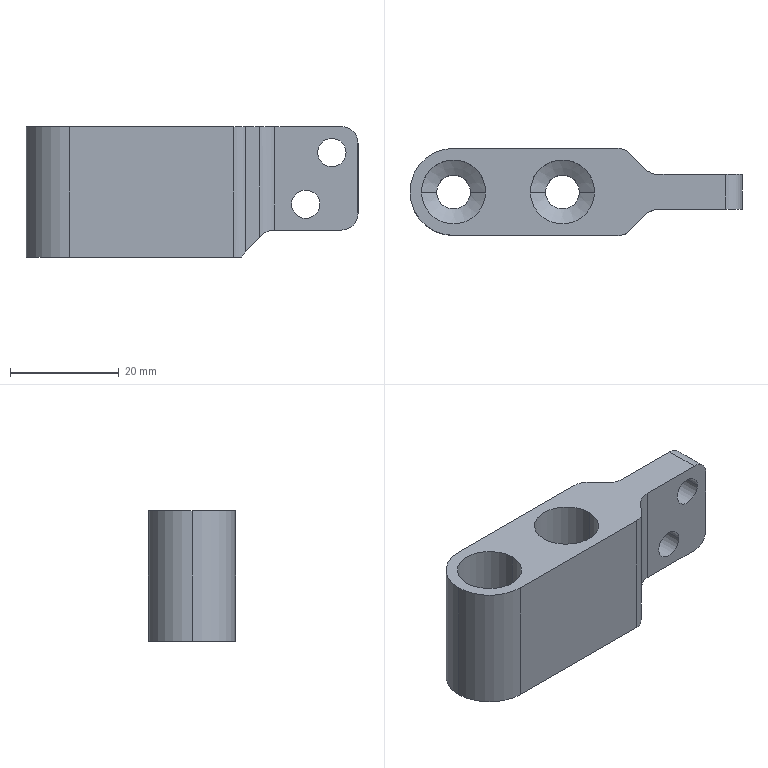Part | NX | 1 solid | 36 faces | box 60.988 x 16 x 24 mm | volume 13127 mm3 | cylinder 21 | plane 11 | cone 4 | commonest cylinder face diameters 5.2 x4 6 x4 6.2 x4 11.8 x4 8 x3 16 x2
STEP:
#1=CARTESIAN_POINT('',(-16.594,0.,-17.));
#2=VERTEX_POINT('',#1);
#3=CARTESIAN_POINT('',(-28.394,0.,-17.));
#4=VERTEX_POINT('',#3);
#5=CARTESIAN_POINT('',(-22.494,0.,-17.));
#6=DIRECTION('',(0.,0.,1.));
#7=DIRECTION('',(-1.,0.,0.));
#8=AXIS2_PLACEMENT_3D('',#5,#6,#7);
#9=CIRCLE('',#8,5.9);
#10=EDGE_CURVE('',#2,#4,#9,.T.);
#11=ORIENTED_EDGE('',*,*,#10,.F.);
#12=CARTESIAN_POINT('',(-16.594,0.,0.));
#13=VERTEX_POINT('',#12);
#14=CARTESIAN_POINT('',(-16.594,0.,0.));
#15=DIRECTION('',(0.,0.,1.));
#16=VECTOR('',#15,1000.);
#17=LINE('',#14,#16);
#18=EDGE_CURVE('',#13,#2,#17,.F.);
#19=ORIENTED_EDGE('',*,*,#18,.F.);
#20=CARTESIAN_POINT('',(-28.394,0.,0.));
#21=VERTEX_POINT('',#20);
#22=CARTESIAN_POINT('',(-22.494,0.,0.));
#23=DIRECTION('',(0.,0.,1.));
#24=DIRECTION('',(-1.,0.,0.));
#25=AXIS2_PLACEMENT_3D('',#22,#23,#24);
#26=CIRCLE('',#25,5.9);
#27=EDGE_CURVE('',#13,#21,#26,.T.);
#28=ORIENTED_EDGE('',*,*,#27,.T.);
#29=CARTESIAN_POINT('',(-28.394,0.,0.));
#30=DIRECTION('',(0.,0.,1.));
#31=VECTOR('',#30,1000.);
#32=LINE('',#29,#31);
#33=EDGE_CURVE('',#21,#4,#32,.F.);
#34=ORIENTED_EDGE('',*,*,#33,.T.);
#35=EDGE_LOOP('',(#11,#19,#28,#34));
#36=FACE_BOUND('',#35,.T.);
#37=CARTESIAN_POINT('',(-22.494,0.,0.));
#38=DIRECTION('',(0.,0.,1.));
#39=DIRECTION('',(1.,0.,0.));
#40=AXIS2_PLACEMENT_3D('',#37,#38,#39);
#41=CYLINDRICAL_SURFACE('',#40,5.9);
#42=ADVANCED_FACE('',(#36),#41,.F.);
#43=CARTESIAN_POINT('',(-19.394,0.,-18.682));
#44=VERTEX_POINT('',#43);
#45=CARTESIAN_POINT('',(-25.594,0.,-18.682));
#46=VERTEX_POINT('',#45);
#47=CARTESIAN_POINT('',(-22.494,0.,-18.682));
#48=DIRECTION('',(0.,0.,1.));
#49=DIRECTION('',(-1.,0.,0.));
#50=AXIS2_PLACEMENT_3D('',#47,#48,#49);
#51=CIRCLE('',#50,3.1);
#52=EDGE_CURVE('',#44,#46,#51,.T.);
#53=ORIENTED_EDGE('',*,*,#52,.F.);
#54=CARTESIAN_POINT('',(-16.594,0.,-17.));
#55=DIRECTION('',(0.8572,0.,0.515));
#56=VECTOR('',#55,1000.);
#57=LINE('',#54,#56);
#58=EDGE_CURVE('',#2,#44,#57,.F.);
#59=ORIENTED_EDGE('',*,*,#58,.F.);
#60=ORIENTED_EDGE('',*,*,#10,.T.);
#61=CARTESIAN_POINT('',(-28.394,0.,-17.));
#62=DIRECTION('',(-0.8572,0.,0.515));
#63=VECTOR('',#62,1000.);
#64=LINE('',#61,#63);
#65=EDGE_CURVE('',#4,#46,#64,.F.);
#66=ORIENTED_EDGE('',*,*,#65,.T.);
#67=EDGE_LOOP('',(#53,#59,#60,#66));
#68=FACE_BOUND('',#67,.T.);
#69=CARTESIAN_POINT('',(-22.494,0.,-17.));
#70=DIRECTION('',(0.,0.,1.));
#71=DIRECTION('',(1.,0.,0.));
#72=AXIS2_PLACEMENT_3D('',#69,#70,#71);
#73=CONICAL_SURFACE('',#72,5.9,1.03);
#74=ADVANCED_FACE('',(#68),#73,.F.);
#75=CARTESIAN_POINT('',(3.406,0.,-17.));
#76=VERTEX_POINT('',#75);
#77=CARTESIAN_POINT('',(-8.394,0.,-17.));
#78=VERTEX_POINT('',#77);
#79=CARTESIAN_POINT('',(-2.494,0.,-17.));
#80=DIRECTION('',(0.,0.,1.));
#81=DIRECTION('',(-1.,0.,0.));
#82=AXIS2_PLACEMENT_3D('',#79,#80,#81);
#83=CIRCLE('',#82,5.9);
#84=EDGE_CURVE('',#76,#78,#83,.T.);
#85=ORIENTED_EDGE('',*,*,#84,.F.);
#86=CARTESIAN_POINT('',(3.406,0.,0.));
#87=VERTEX_POINT('',#86);
#88=CARTESIAN_POINT('',(3.406,0.,0.));
#89=DIRECTION('',(0.,0.,1.));
#90=VECTOR('',#89,1000.);
#91=LINE('',#88,#90);
#92=EDGE_CURVE('',#87,#76,#91,.F.);
#93=ORIENTED_EDGE('',*,*,#92,.F.);
#94=CARTESIAN_POINT('',(-8.394,0.,0.));
#95=VERTEX_POINT('',#94);
#96=CARTESIAN_POINT('',(-2.494,0.,0.));
#97=DIRECTION('',(0.,0.,1.));
#98=DIRECTION('',(-1.,0.,0.));
#99=AXIS2_PLACEMENT_3D('',#96,#97,#98);
#100=CIRCLE('',#99,5.9);
#101=EDGE_CURVE('',#87,#95,#100,.T.);
#102=ORIENTED_EDGE('',*,*,#101,.T.);
#103=CARTESIAN_POINT('',(-8.394,0.,0.));
#104=DIRECTION('',(0.,0.,1.));
#105=VECTOR('',#104,1000.);
#106=LINE('',#103,#105);
#107=EDGE_CURVE('',#95,#78,#106,.F.);
#108=ORIENTED_EDGE('',*,*,#107,.T.);
#109=EDGE_LOOP('',(#85,#93,#102,#108));
#110=FACE_BOUND('',#109,.T.);
#111=CARTESIAN_POINT('',(-2.494,0.,0.));
#112=DIRECTION('',(0.,0.,1.));
#113=DIRECTION('',(1.,0.,0.));
#114=AXIS2_PLACEMENT_3D('',#111,#112,#113);
#115=CYLINDRICAL_SURFACE('',#114,5.9);
#116=ADVANCED_FACE('',(#110),#115,.F.);
#117=CARTESIAN_POINT('',(0.6061,0.,-18.682));
#118=VERTEX_POINT('',#117);
#119=CARTESIAN_POINT('',(-5.594,0.,-18.682));
#120=VERTEX_POINT('',#119);
#121=CARTESIAN_POINT('',(-2.494,0.,-18.682));
#122=DIRECTION('',(0.,0.,1.));
#123=DIRECTION('',(-1.,0.,0.));
#124=AXIS2_PLACEMENT_3D('',#121,#122,#123);
#125=CIRCLE('',#124,3.1);
#126=EDGE_CURVE('',#118,#120,#125,.T.);
#127=ORIENTED_EDGE('',*,*,#126,.F.);
#128=CARTESIAN_POINT('',(3.406,0.,-17.));
#129=DIRECTION('',(0.8572,0.,0.515));
#130=VECTOR('',#129,1000.);
#131=LINE('',#128,#130);
#132=EDGE_CURVE('',#76,#118,#131,.F.);
#133=ORIENTED_EDGE('',*,*,#132,.F.);
#134=ORIENTED_EDGE('',*,*,#84,.T.);
#135=CARTESIAN_POINT('',(-8.394,0.,-17.));
#136=DIRECTION('',(-0.8572,0.,0.515));
#137=VECTOR('',#136,1000.);
#138=LINE('',#135,#137);
#139=EDGE_CURVE('',#78,#120,#138,.F.);
#140=ORIENTED_EDGE('',*,*,#139,.T.);
#141=EDGE_LOOP('',(#127,#133,#134,#140));
#142=FACE_BOUND('',#141,.T.);
#143=CARTESIAN_POINT('',(-2.494,0.,-17.));
#144=DIRECTION('',(0.,0.,1.));
#145=DIRECTION('',(1.,0.,0.));
#146=AXIS2_PLACEMENT_3D('',#143,#144,#145);
#147=CONICAL_SURFACE('',#146,5.9,1.03);
#148=ADVANCED_FACE('',(#142),#147,.F.);
#149=CARTESIAN_POINT('',(-30.494,0.,-24.));
#150=VERTEX_POINT('',#149);
#151=CARTESIAN_POINT('',(-22.494,8.,-24.));
#152=VERTEX_POINT('',#151);
#153=CARTESIAN_POINT('',(-22.494,0.,-24.));
#154=DIRECTION('',(0.,0.,-1.));
#155=DIRECTION('',(-1.,0.,0.));
#156=AXIS2_PLACEMENT_3D('',#153,#154,#155);
#157=CIRCLE('',#156,8.);
#158=EDGE_CURVE('',#150,#152,#157,.T.);
#159=ORIENTED_EDGE('',*,*,#158,.F.);
#160=CARTESIAN_POINT('',(-30.494,0.,0.));
#161=VERTEX_POINT('',#160);
#162=CARTESIAN_POINT('',(-30.494,0.,-24.06));
#163=DIRECTION('',(0.,0.,1.));
#164=VECTOR('',#163,1000.);
#165=LINE('',#162,#164);
#166=EDGE_CURVE('',#150,#161,#165,.T.);
#167=ORIENTED_EDGE('',*,*,#166,.T.);
#168=CARTESIAN_POINT('',(-22.494,8.,0.));
#169=VERTEX_POINT('',#168);
#170=CARTESIAN_POINT('',(-22.494,0.,0.));
#171=DIRECTION('',(0.,0.,-1.));
#172=DIRECTION('',(-1.,0.,0.));
#173=AXIS2_PLACEMENT_3D('',#170,#171,#172);
#174=CIRCLE('',#173,8.);
#175=EDGE_CURVE('',#161,#169,#174,.T.);
#176=ORIENTED_EDGE('',*,*,#175,.T.);
#177=CARTESIAN_POINT('',(-22.494,8.,-3.));
#178=DIRECTION('',(0.,0.,-1.));
#179=VECTOR('',#178,1000.);
#180=LINE('',#177,#179);
#181=EDGE_CURVE('',#169,#152,#180,.T.);
#182=ORIENTED_EDGE('',*,*,#181,.T.);
#183=EDGE_LOOP('',(#159,#167,#176,#182));
#184=FACE_BOUND('',#183,.T.);
#185=CARTESIAN_POINT('',(-22.494,0.,-24.06));
#186=DIRECTION('',(0.,0.,1.));
#187=DIRECTION('',(1.,0.,0.));
#188=AXIS2_PLACEMENT_3D('',#185,#186,#187);
#189=CYLINDRICAL_SURFACE('',#188,8.);
#190=ADVANCED_FACE('',(#184),#189,.T.);
#191=CARTESIAN_POINT('',(0.6061,0.,-24.));
#192=VERTEX_POINT('',#191);
#193=CARTESIAN_POINT('',(-5.594,0.,-24.));
#194=VERTEX_POINT('',#193);
#195=CARTESIAN_POINT('',(-2.494,0.,-24.));
#196=DIRECTION('',(0.,0.,1.));
#197=DIRECTION('',(-1.,0.,0.));
#198=AXIS2_PLACEMENT_3D('',#195,#196,#197);
#199=CIRCLE('',#198,3.1);
#200=EDGE_CURVE('',#192,#194,#199,.T.);
#201=ORIENTED_EDGE('',*,*,#200,.F.);
#202=CARTESIAN_POINT('',(0.6061,0.,-24.06));
#203=DIRECTION('',(0.,0.,1.));
#204=VECTOR('',#203,1000.);
#205=LINE('',#202,#204);
#206=EDGE_CURVE('',#118,#192,#205,.F.);
#207=ORIENTED_EDGE('',*,*,#206,.F.);
#208=ORIENTED_EDGE('',*,*,#126,.T.);
#209=CARTESIAN_POINT('',(-5.594,0.,-24.06));
#210=DIRECTION('',(0.,0.,1.));
#211=VECTOR('',#210,1000.);
#212=LINE('',#209,#211);
#213=EDGE_CURVE('',#120,#194,#212,.F.);
#214=ORIENTED_EDGE('',*,*,#213,.T.);
#215=EDGE_LOOP('',(#201,#207,#208,#214));
#216=FACE_BOUND('',#215,.T.);
#217=CARTESIAN_POINT('',(-2.494,0.,-24.06));
#218=DIRECTION('',(0.,0.,1.));
#219=DIRECTION('',(1.,0.,0.));
#220=AXIS2_PLACEMENT_3D('',#217,#218,#219);
#221=CYLINDRICAL_SURFACE('',#220,3.1);
#222=ADVANCED_FACE('',(#216),#221,.F.);
#223=CARTESIAN_POINT('',(23.494,3.2,-14.252));
#224=VERTEX_POINT('',#223);
#225=CARTESIAN_POINT('',(18.294,3.2,-14.252));
#226=VERTEX_POINT('',#225);
#227=CARTESIAN_POINT('',(20.894,3.2,-14.252));
#228=DIRECTION('',(0.,1.,0.));
#229=DIRECTION('',(1.,0.,0.));
#230=AXIS2_PLACEMENT_3D('',#227,#228,#229);
#231=CIRCLE('',#230,2.6);
#232=EDGE_CURVE('',#224,#226,#231,.T.);
#233=ORIENTED_EDGE('',*,*,#232,.T.);
#234=CARTESIAN_POINT('',(18.294,-3.2,-14.252));
#235=VERTEX_POINT('',#234);
#236=CARTESIAN_POINT('',(18.294,8.,-14.252));
#237=DIRECTION('',(0.,-1.,0.));
#238=VECTOR('',#237,1000.);
#239=LINE('',#236,#238);
#240=EDGE_CURVE('',#235,#226,#239,.F.);
#241=ORIENTED_EDGE('',*,*,#240,.F.);
#242=CARTESIAN_POINT('',(23.494,-3.2,-14.252));
#243=VERTEX_POINT('',#242);
#244=CARTESIAN_POINT('',(20.894,-3.2,-14.252));
#245=DIRECTION('',(0.,-1.,0.));
#246=DIRECTION('',(1.,0.,0.));
#247=AXIS2_PLACEMENT_3D('',#244,#245,#246);
#248=CIRCLE('',#247,2.6);
#249=EDGE_CURVE('',#235,#243,#248,.T.);
#250=ORIENTED_EDGE('',*,*,#249,.T.);
#251=CARTESIAN_POINT('',(23.494,8.,-14.252));
#252=DIRECTION('',(0.,-1.,0.));
#253=VECTOR('',#252,1000.);
#254=LINE('',#251,#253);
#255=EDGE_CURVE('',#243,#224,#254,.F.);
#256=ORIENTED_EDGE('',*,*,#255,.T.);
#257=EDGE_LOOP('',(#233,#241,#250,#256));
#258=FACE_BOUND('',#257,.T.);
#259=CARTESIAN_POINT('',(20.894,8.,-14.252));
#260=DIRECTION('',(0.,-1.,0.));
#261=DIRECTION('',(-1.,0.,0.));
#262=AXIS2_PLACEMENT_3D('',#259,#260,#261);
#263=CYLINDRICAL_SURFACE('',#262,2.6);
#264=ADVANCED_FACE('',(#258),#263,.F.);
#265=CARTESIAN_POINT('',(28.294,3.2,-4.752));
#266=VERTEX_POINT('',#265);
#267=CARTESIAN_POINT('',(23.094,3.2,-4.752));
#268=VERTEX_POINT('',#267);
#269=CARTESIAN_POINT('',(25.694,3.2,-4.752));
#270=DIRECTION('',(0.,1.,0.));
#271=DIRECTION('',(1.,0.,0.));
#272=AXIS2_PLACEMENT_3D('',#269,#270,#271);
#273=CIRCLE('',#272,2.6);
#274=EDGE_CURVE('',#266,#268,#273,.T.);
#275=ORIENTED_EDGE('',*,*,#274,.T.);
#276=CARTESIAN_POINT('',(23.094,-3.2,-4.752));
#277=VERTEX_POINT('',#276);
#278=CARTESIAN_POINT('',(23.094,8.,-4.752));
#279=DIRECTION('',(0.,-1.,0.));
#280=VECTOR('',#279,1000.);
#281=LINE('',#278,#280);
#282=EDGE_CURVE('',#277,#268,#281,.F.);
#283=ORIENTED_EDGE('',*,*,#282,.F.);
#284=CARTESIAN_POINT('',(28.294,-3.2,-4.752));
#285=VERTEX_POINT('',#284);
#286=CARTESIAN_POINT('',(25.694,-3.2,-4.752));
#287=DIRECTION('',(0.,-1.,0.));
#288=DIRECTION('',(1.,0.,0.));
#289=AXIS2_PLACEMENT_3D('',#286,#287,#288);
#290=CIRCLE('',#289,2.6);
#291=EDGE_CURVE('',#277,#285,#290,.T.);
#292=ORIENTED_EDGE('',*,*,#291,.T.);
#293=CARTESIAN_POINT('',(28.294,8.,-4.752));
#294=DIRECTION('',(0.,-1.,0.));
#295=VECTOR('',#294,1000.);
#296=LINE('',#293,#295);
#297=EDGE_CURVE('',#285,#266,#296,.F.);
#298=ORIENTED_EDGE('',*,*,#297,.T.);
#299=EDGE_LOOP('',(#275,#283,#292,#298));
#300=FACE_BOUND('',#299,.T.);
#301=CARTESIAN_POINT('',(25.694,8.,-4.752));
#302=DIRECTION('',(0.,-1.,0.));
#303=DIRECTION('',(-1.,0.,0.));
#304=AXIS2_PLACEMENT_3D('',#301,#302,#303);
#305=CYLINDRICAL_SURFACE('',#304,2.6);
#306=ADVANCED_FACE('',(#300),#305,.F.);
#307=CARTESIAN_POINT('',(-19.394,0.,-24.));
#308=VERTEX_POINT('',#307);
#309=CARTESIAN_POINT('',(-25.594,0.,-24.));
#310=VERTEX_POINT('',#309);
#311=CARTESIAN_POINT('',(-22.494,0.,-24.));
#312=DIRECTION('',(0.,0.,1.));
#313=DIRECTION('',(-1.,0.,0.));
#314=AXIS2_PLACEMENT_3D('',#311,#312,#313);
#315=CIRCLE('',#314,3.1);
#316=EDGE_CURVE('',#308,#310,#315,.T.);
#317=ORIENTED_EDGE('',*,*,#316,.F.);
#318=CARTESIAN_POINT('',(-19.394,0.,-24.06));
#319=DIRECTION('',(0.,0.,1.));
#320=VECTOR('',#319,1000.);
#321=LINE('',#318,#320);
#322=EDGE_CURVE('',#44,#308,#321,.F.);
#323=ORIENTED_EDGE('',*,*,#322,.F.);
#324=ORIENTED_EDGE('',*,*,#52,.T.);
#325=CARTESIAN_POINT('',(-25.594,0.,-24.06));
#326=DIRECTION('',(0.,0.,1.));
#327=VECTOR('',#326,1000.);
#328=LINE('',#325,#327);
#329=EDGE_CURVE('',#46,#310,#328,.F.);
#330=ORIENTED_EDGE('',*,*,#329,.T.);
#331=EDGE_LOOP('',(#317,#323,#324,#330));
#332=FACE_BOUND('',#331,.T.);
#333=CARTESIAN_POINT('',(-22.494,0.,-24.06));
#334=DIRECTION('',(0.,0.,1.));
#335=DIRECTION('',(1.,0.,0.));
#336=AXIS2_PLACEMENT_3D('',#333,#334,#335);
#337=CYLINDRICAL_SURFACE('',#336,3.1);
#338=ADVANCED_FACE('',(#332),#337,.F.);
#339=ORIENTED_EDGE('',*,*,#322,.T.);
#340=CARTESIAN_POINT('',(-22.494,0.,-24.));
#341=DIRECTION('',(0.,0.,1.));
#342=DIRECTION('',(-1.,0.,0.));
#343=AXIS2_PLACEMENT_3D('',#340,#341,#342);
#344=CIRCLE('',#343,3.1);
#345=EDGE_CURVE('',#310,#308,#344,.T.);
#346=ORIENTED_EDGE('',*,*,#345,.F.);
#347=ORIENTED_EDGE('',*,*,#329,.F.);
#348=CARTESIAN_POINT('',(-22.494,0.,-18.682));
#349=DIRECTION('',(0.,0.,1.));
#350=DIRECTION('',(-1.,0.,0.));
#351=AXIS2_PLACEMENT_3D('',#348,#349,#350);
#352=CIRCLE('',#351,3.1);
#353=EDGE_CURVE('',#46,#44,#352,.T.);
#354=ORIENTED_EDGE('',*,*,#353,.T.);
#355=EDGE_LOOP('',(#339,#346,#347,#354));
#356=FACE_BOUND('',#355,.T.);
#357=CARTESIAN_POINT('',(-22.494,0.,-24.06));
#358=DIRECTION('',(0.,0.,1.));
#359=DIRECTION('',(1.,0.,0.));
#360=AXIS2_PLACEMENT_3D('',#357,#358,#359);
#361=CYLINDRICAL_SURFACE('',#360,3.1);
#362=ADVANCED_FACE('',(#356),#361,.F.);
#363=CARTESIAN_POINT('',(-22.494,-8.,0.));
#364=VERTEX_POINT('',#363);
#365=CARTESIAN_POINT('',(-22.494,-8.,-24.));
#366=VERTEX_POINT('',#365);
#367=CARTESIAN_POINT('',(-22.494,-8.,-3.));
#368=DIRECTION('',(0.,0.,-1.));
#369=VECTOR('',#368,1000.);
#370=LINE('',#367,#369);
#371=EDGE_CURVE('',#364,#366,#370,.T.);
#372=ORIENTED_EDGE('',*,*,#371,.T.);
#373=CARTESIAN_POINT('',(7.706,-8.,-24.));
#374=VERTEX_POINT('',#373);
#375=CARTESIAN_POINT('',(27.506,-8.,-24.));
#376=DIRECTION('',(1.,0.,0.));
#377=VECTOR('',#376,1000.);
#378=LINE('',#375,#377);
#379=EDGE_CURVE('',#366,#374,#378,.T.);
#380=ORIENTED_EDGE('',*,*,#379,.T.);
#381=CARTESIAN_POINT('',(7.706,-8.,0.));
#382=VERTEX_POINT('',#381);
#383=CARTESIAN_POINT('',(7.706,-8.,-3.));
#384=DIRECTION('',(0.,0.,1.));
#385=VECTOR('',#384,1000.);
#386=LINE('',#383,#385);
#387=EDGE_CURVE('',#374,#382,#386,.T.);
#388=ORIENTED_EDGE('',*,*,#387,.T.);
#389=CARTESIAN_POINT('',(27.506,-8.,0.));
#390=DIRECTION('',(-1.,0.,0.));
#391=VECTOR('',#390,1000.);
#392=LINE('',#389,#391);
#393=EDGE_CURVE('',#382,#364,#392,.T.);
#394=ORIENTED_EDGE('',*,*,#393,.T.);
#395=EDGE_LOOP('',(#372,#380,#388,#394));
#396=FACE_BOUND('',#395,.T.);
#397=CARTESIAN_POINT('',(27.506,-8.,-3.));
#398=DIRECTION('',(0.,-1.,0.));
#399=DIRECTION('',(-1.,0.,0.));
#400=AXIS2_PLACEMENT_3D('',#397,#398,#399);
#401=PLANE('',#400);
#402=ADVANCED_FACE('',(#396),#401,.T.);
#403=ORIENTED_EDGE('',*,*,#345,.T.);
#404=ORIENTED_EDGE('',*,*,#316,.T.);
#405=EDGE_LOOP('',(#403,#404));
#406=FACE_BOUND('',#405,.T.);
#407=CARTESIAN_POINT('',(-22.494,0.,-24.));
#408=DIRECTION('',(0.,0.,-1.));
#409=DIRECTION('',(-1.,0.,0.));
#410=AXIS2_PLACEMENT_3D('',#407,#408,#409);
#411=CIRCLE('',#410,8.);
#412=EDGE_CURVE('',#366,#150,#411,.T.);
#413=ORIENTED_EDGE('',*,*,#412,.T.);
#414=ORIENTED_EDGE('',*,*,#158,.T.);
#415=CARTESIAN_POINT('',(7.706,8.,-24.));
#416=VERTEX_POINT('',#415);
#417=CARTESIAN_POINT('',(-30.494,8.,-24.));
#418=DIRECTION('',(1.,0.,0.));
#419=VECTOR('',#418,1000.);
#420=LINE('',#417,#419);
#421=EDGE_CURVE('',#152,#416,#420,.T.);
#422=ORIENTED_EDGE('',*,*,#421,.T.);
#423=CARTESIAN_POINT('',(9.006,7.704,-24.));
#424=VERTEX_POINT('',#423);
#425=CARTESIAN_POINT('',(7.706,5.,-24.));
#426=DIRECTION('',(0.,0.,1.));
#427=DIRECTION('',(-1.,0.,0.));
#428=AXIS2_PLACEMENT_3D('',#425,#426,#427);
#429=CIRCLE('',#428,3.);
#430=EDGE_CURVE('',#424,#416,#429,.T.);
#431=ORIENTED_EDGE('',*,*,#430,.F.);
#432=CARTESIAN_POINT('',(9.006,-7.704,-24.));
#433=VERTEX_POINT('',#432);
#434=CARTESIAN_POINT('',(9.006,8.,-24.));
#435=DIRECTION('',(0.,-1.,0.));
#436=VECTOR('',#435,1000.);
#437=LINE('',#434,#436);
#438=EDGE_CURVE('',#424,#433,#437,.T.);
#439=ORIENTED_EDGE('',*,*,#438,.T.);
#440=CARTESIAN_POINT('',(7.706,-5.,-24.));
#441=DIRECTION('',(0.,0.,-1.));
#442=DIRECTION('',(-1.,0.,0.));
#443=AXIS2_PLACEMENT_3D('',#440,#441,#442);
#444=CIRCLE('',#443,3.);
#445=EDGE_CURVE('',#433,#374,#444,.T.);
#446=ORIENTED_EDGE('',*,*,#445,.T.);
#447=ORIENTED_EDGE('',*,*,#379,.F.);
#448=EDGE_LOOP('',(#413,#414,#422,#431,#439,#446,#447));
#449=FACE_BOUND('',#448,.T.);
#450=CARTESIAN_POINT('',(-2.494,0.,-24.));
#451=DIRECTION('',(0.,0.,1.));
#452=DIRECTION('',(-1.,0.,0.));
#453=AXIS2_PLACEMENT_3D('',#450,#451,#452);
#454=CIRCLE('',#453,3.1);
#455=EDGE_CURVE('',#194,#192,#454,.T.);
#456=ORIENTED_EDGE('',*,*,#455,.T.);
#457=ORIENTED_EDGE('',*,*,#200,.T.);
#458=EDGE_LOOP('',(#456,#457));
#459=FACE_BOUND('',#458,.T.);
#460=CARTESIAN_POINT('',(-30.494,8.,-24.));
#461=DIRECTION('',(0.,0.,-1.));
#462=DIRECTION('',(-1.,0.,0.));
#463=AXIS2_PLACEMENT_3D('',#460,#461,#462);
#464=PLANE('',#463);
#465=ADVANCED_FACE('',(#406,#449,#459),#464,.T.);
#466=ORIENTED_EDGE('',*,*,#166,.F.);
#467=ORIENTED_EDGE('',*,*,#412,.F.);
#468=ORIENTED_EDGE('',*,*,#371,.F.);
#469=CARTESIAN_POINT('',(-22.494,0.,0.));
#470=DIRECTION('',(0.,0.,-1.));
#471=DIRECTION('',(-1.,0.,0.));
#472=AXIS2_PLACEMENT_3D('',#469,#470,#471);
#473=CIRCLE('',#472,8.);
#474=EDGE_CURVE('',#364,#161,#473,.T.);
#475=ORIENTED_EDGE('',*,*,#474,.T.);
#476=EDGE_LOOP('',(#466,#467,#468,#475));
#477=FACE_BOUND('',#476,.T.);
#478=CARTESIAN_POINT('',(-22.494,0.,-24.06));
#479=DIRECTION('',(0.,0.,1.));
#480=DIRECTION('',(1.,0.,0.));
#481=AXIS2_PLACEMENT_3D('',#478,#479,#480);
#482=CYLINDRICAL_SURFACE('',#481,8.);
#483=ADVANCED_FACE('',(#477),#482,.T.);
#484=CARTESIAN_POINT('',(-22.494,0.,0.));
#485=DIRECTION('',(0.,0.,1.));
#486=DIRECTION('',(-1.,0.,0.));
#487=AXIS2_PLACEMENT_3D('',#484,#485,#486);
#488=CIRCLE('',#487,5.9);
#489=EDGE_CURVE('',#21,#13,#488,.T.);
#490=ORIENTED_EDGE('',*,*,#489,.F.);
#491=ORIENTED_EDGE('',*,*,#27,.F.);
#492=EDGE_LOOP('',(#490,#491));
#493=FACE_BOUND('',#492,.T.);
#494=CARTESIAN_POINT('',(-2.494,0.,0.));
#495=DIRECTION('',(0.,0.,1.));
#496=DIRECTION('',(-1.,0.,0.));
#497=AXIS2_PLACEMENT_3D('',#494,#495,#496);
#498=CIRCLE('',#497,5.9);
#499=EDGE_CURVE('',#95,#87,#498,.T.);
#500=ORIENTED_EDGE('',*,*,#499,.F.);
#501=ORIENTED_EDGE('',*,*,#101,.F.);
#502=EDGE_LOOP('',(#500,#501));
#503=FACE_BOUND('',#502,.T.);
#504=CARTESIAN_POINT('',(15.239,-3.2,0.));
#505=VERTEX_POINT('',#504);
#506=CARTESIAN_POINT('',(27.494,-3.2,0.));
#507=VERTEX_POINT('',#506);
#508=CARTESIAN_POINT('',(30.506,-3.2,0.));
#509=DIRECTION('',(1.,0.,0.));
#510=VECTOR('',#509,1000.);
#511=LINE('',#508,#510);
#512=EDGE_CURVE('',#505,#507,#511,.T.);
#513=ORIENTED_EDGE('',*,*,#512,.T.);
#514=CARTESIAN_POINT('',(27.494,3.2,0.));
#515=VERTEX_POINT('',#514);
#516=CARTESIAN_POINT('',(27.494,3.2,0.));
#517=DIRECTION('',(0.,1.,0.));
#518=VECTOR('',#517,1000.);
#519=LINE('',#516,#518);
#520=EDGE_CURVE('',#507,#515,#519,.T.);
#521=ORIENTED_EDGE('',*,*,#520,.T.);
#522=CARTESIAN_POINT('',(15.239,3.2,0.));
#523=VERTEX_POINT('',#522);
#524=CARTESIAN_POINT('',(15.239,3.2,0.));
#525=DIRECTION('',(-1.,0.,0.));
#526=VECTOR('',#525,1000.);
#527=LINE('',#524,#526);
#528=EDGE_CURVE('',#515,#523,#527,.T.);
#529=ORIENTED_EDGE('',*,*,#528,.T.);
#530=CARTESIAN_POINT('',(12.321,4.464,0.));
#531=VERTEX_POINT('',#530);
#532=CARTESIAN_POINT('',(15.239,7.2,0.));
#533=DIRECTION('',(0.,0.,1.));
#534=DIRECTION('',(1.,0.,0.));
#535=AXIS2_PLACEMENT_3D('',#532,#533,#534);
#536=CIRCLE('',#535,4.);
#537=EDGE_CURVE('',#523,#531,#536,.F.);
#538=ORIENTED_EDGE('',*,*,#537,.T.);
#539=CARTESIAN_POINT('',(9.895,7.052,0.));
#540=VERTEX_POINT('',#539);
#541=CARTESIAN_POINT('',(9.895,7.052,0.));
#542=DIRECTION('',(-0.6839,0.7295,0.));
#543=VECTOR('',#542,1000.);
#544=LINE('',#541,#543);
#545=EDGE_CURVE('',#531,#540,#544,.T.);
#546=ORIENTED_EDGE('',*,*,#545,.T.);
#547=CARTESIAN_POINT('',(7.706,8.,0.));
#548=VERTEX_POINT('',#547);
#549=CARTESIAN_POINT('',(7.706,5.,0.));
#550=DIRECTION('',(0.,0.,1.));
#551=DIRECTION('',(-1.,0.,0.));
#552=AXIS2_PLACEMENT_3D('',#549,#550,#551);
#553=CIRCLE('',#552,3.);
#554=EDGE_CURVE('',#540,#548,#553,.T.);
#555=ORIENTED_EDGE('',*,*,#554,.T.);
#556=CARTESIAN_POINT('',(27.506,8.,0.));
#557=DIRECTION('',(-1.,0.,0.));
#558=VECTOR('',#557,1000.);
#559=LINE('',#556,#558);
#560=EDGE_CURVE('',#548,#169,#559,.T.);
#561=ORIENTED_EDGE('',*,*,#560,.T.);
#562=ORIENTED_EDGE('',*,*,#175,.F.);
#563=ORIENTED_EDGE('',*,*,#474,.F.);
#564=ORIENTED_EDGE('',*,*,#393,.F.);
#565=CARTESIAN_POINT('',(9.895,-7.052,0.));
#566=VERTEX_POINT('',#565);
#567=CARTESIAN_POINT('',(7.706,-5.,0.));
#568=DIRECTION('',(0.,0.,1.));
#569=DIRECTION('',(-1.,0.,0.));
#570=AXIS2_PLACEMENT_3D('',#567,#568,#569);
#571=CIRCLE('',#570,3.);
#572=EDGE_CURVE('',#382,#566,#571,.T.);
#573=ORIENTED_EDGE('',*,*,#572,.T.);
#574=CARTESIAN_POINT('',(12.321,-4.464,0.));
#575=VERTEX_POINT('',#574);
#576=CARTESIAN_POINT('',(12.321,-4.464,0.));
#577=DIRECTION('',(0.6839,0.7295,0.));
#578=VECTOR('',#577,1000.);
#579=LINE('',#576,#578);
#580=EDGE_CURVE('',#566,#575,#579,.T.);
#581=ORIENTED_EDGE('',*,*,#580,.T.);
#582=CARTESIAN_POINT('',(15.239,-7.2,0.));
#583=DIRECTION('',(0.,0.,1.));
#584=DIRECTION('',(1.,0.,0.));
#585=AXIS2_PLACEMENT_3D('',#582,#583,#584);
#586=CIRCLE('',#585,4.);
#587=EDGE_CURVE('',#575,#505,#586,.F.);
#588=ORIENTED_EDGE('',*,*,#587,.T.);
#589=EDGE_LOOP('',(#513,#521,#529,#538,#546,#555,#561,#562,#563,#564,#573,#581,#588));
#590=FACE_BOUND('',#589,.T.);
#591=CARTESIAN_POINT('',(27.506,8.,0.));
#592=DIRECTION('',(0.,0.,1.));
#593=DIRECTION('',(1.,0.,0.));
#594=AXIS2_PLACEMENT_3D('',#591,#592,#593);
#595=PLANE('',#594);
#596=ADVANCED_FACE('',(#493,#503,#590),#595,.T.);
#597=CARTESIAN_POINT('',(9.895,-7.052,-23.012));
#598=VERTEX_POINT('',#597);
#599=CARTESIAN_POINT('',(9.895,-7.052,-24.06));
#600=DIRECTION('',(0.,0.,1.));
#601=VECTOR('',#600,1000.);
#602=LINE('',#599,#601);
#603=EDGE_CURVE('',#598,#566,#602,.T.);
#604=ORIENTED_EDGE('',*,*,#603,.T.);
#605=ORIENTED_EDGE('',*,*,#572,.F.);
#606=ORIENTED_EDGE('',*,*,#387,.F.);
#607=ORIENTED_EDGE('',*,*,#445,.F.);
#608=CARTESIAN_POINT('',(9.006,-7.704,-24.));
#609=CARTESIAN_POINT('',(9.341,-7.543,-23.628));
#610=CARTESIAN_POINT('',(9.641,-7.323,-23.295));
#611=CARTESIAN_POINT('',(9.895,-7.052,-23.012));
#612=(BOUNDED_CURVE()B_SPLINE_CURVE(3,(#608,#609,#610,#611),.UNSPECIFIED.,.F.,.F.)B_SPLINE_CURVE_WITH_KNOTS((4,4),(0.,1.),.PIECEWISE_BEZIER_KNOTS.)CURVE()GEOMETRIC_REPRESENTATION_ITEM()RATIONAL_B_SPLINE_CURVE((1.,0.9887,0.9887,1.))REPRESENTATION_ITEM(''));
#613=EDGE_CURVE('',#433,#598,#612,.T.);
#614=ORIENTED_EDGE('',*,*,#613,.T.);
#615=EDGE_LOOP('',(#604,#605,#606,#607,#614));
#616=FACE_BOUND('',#615,.T.);
#617=CARTESIAN_POINT('',(7.706,-5.,-24.06));
#618=DIRECTION('',(0.,0.,1.));
#619=DIRECTION('',(1.,0.,0.));
#620=AXIS2_PLACEMENT_3D('',#617,#618,#619);
#621=CYLINDRICAL_SURFACE('',#620,3.);
#622=ADVANCED_FACE('',(#616),#621,.T.);
#623=CARTESIAN_POINT('',(7.706,8.,-3.));
#624=DIRECTION('',(0.,0.,1.));
#625=VECTOR('',#624,1000.);
#626=LINE('',#623,#625);
#627=EDGE_CURVE('',#416,#548,#626,.T.);
#628=ORIENTED_EDGE('',*,*,#627,.F.);
#629=ORIENTED_EDGE('',*,*,#421,.F.);
#630=ORIENTED_EDGE('',*,*,#181,.F.);
#631=ORIENTED_EDGE('',*,*,#560,.F.);
#632=EDGE_LOOP('',(#628,#629,#630,#631));
#633=FACE_BOUND('',#632,.T.);
#634=CARTESIAN_POINT('',(27.506,8.,-3.));
#635=DIRECTION('',(0.,-1.,0.));
#636=DIRECTION('',(-1.,0.,0.));
#637=AXIS2_PLACEMENT_3D('',#634,#635,#636);
#638=PLANE('',#637);
#639=ADVANCED_FACE('',(#633),#638,.F.);
#640=ORIENTED_EDGE('',*,*,#613,.F.);
#641=ORIENTED_EDGE('',*,*,#438,.F.);
#642=CARTESIAN_POINT('',(9.895,7.052,-23.012));
#643=VERTEX_POINT('',#642);
#644=CARTESIAN_POINT('',(9.006,7.704,-24.));
#645=CARTESIAN_POINT('',(9.341,7.543,-23.628));
#646=CARTESIAN_POINT('',(9.641,7.323,-23.295));
#647=CARTESIAN_POINT('',(9.895,7.052,-23.012));
#648=(BOUNDED_CURVE()B_SPLINE_CURVE(3,(#644,#645,#646,#647),.UNSPECIFIED.,.F.,.F.)B_SPLINE_CURVE_WITH_KNOTS((4,4),(0.,1.),.PIECEWISE_BEZIER_KNOTS.)CURVE()GEOMETRIC_REPRESENTATION_ITEM()RATIONAL_B_SPLINE_CURVE((1.,0.9887,0.9887,1.))REPRESENTATION_ITEM(''));
#649=EDGE_CURVE('',#424,#643,#648,.T.);
#650=ORIENTED_EDGE('',*,*,#649,.T.);
#651=CARTESIAN_POINT('',(12.314,4.471,-20.324));
#652=VERTEX_POINT('',#651);
#653=CARTESIAN_POINT('',(9.895,7.052,-23.012));
#654=DIRECTION('',(0.5445,-0.5808,0.6051));
#655=VECTOR('',#654,1000.);
#656=LINE('',#653,#655);
#657=EDGE_CURVE('',#643,#652,#656,.T.);
#658=ORIENTED_EDGE('',*,*,#657,.T.);
#659=CARTESIAN_POINT('',(12.314,-4.471,-20.324));
#660=VERTEX_POINT('',#659);
#661=CARTESIAN_POINT('',(12.314,8.,-20.324));
#662=DIRECTION('',(0.,-1.,0.));
#663=VECTOR('',#662,1000.);
#664=LINE('',#661,#663);
#665=EDGE_CURVE('',#652,#660,#664,.T.);
#666=ORIENTED_EDGE('',*,*,#665,.T.);
#667=CARTESIAN_POINT('',(12.314,-4.471,-20.324));
#668=DIRECTION('',(-0.5445,-0.5808,-0.6051));
#669=VECTOR('',#668,1000.);
#670=LINE('',#667,#669);
#671=EDGE_CURVE('',#660,#598,#670,.T.);
#672=ORIENTED_EDGE('',*,*,#671,.T.);
#673=EDGE_LOOP('',(#640,#641,#650,#658,#666,#672));
#674=FACE_BOUND('',#673,.T.);
#675=CARTESIAN_POINT('',(9.006,8.,-24.));
#676=DIRECTION('',(0.7433,0.,-0.669));
#677=DIRECTION('',(-0.669,0.,-0.7433));
#678=AXIS2_PLACEMENT_3D('',#675,#676,#677);
#679=PLANE('',#678);
#680=ADVANCED_FACE('',(#674),#679,.T.);
#681=ORIENTED_EDGE('',*,*,#206,.T.);
#682=ORIENTED_EDGE('',*,*,#455,.F.);
#683=ORIENTED_EDGE('',*,*,#213,.F.);
#684=CARTESIAN_POINT('',(-2.494,0.,-18.682));
#685=DIRECTION('',(0.,0.,1.));
#686=DIRECTION('',(-1.,0.,0.));
#687=AXIS2_PLACEMENT_3D('',#684,#685,#686);
#688=CIRCLE('',#687,3.1);
#689=EDGE_CURVE('',#120,#118,#688,.T.);
#690=ORIENTED_EDGE('',*,*,#689,.T.);
#691=EDGE_LOOP('',(#681,#682,#683,#690));
#692=FACE_BOUND('',#691,.T.);
#693=CARTESIAN_POINT('',(-2.494,0.,-24.06));
#694=DIRECTION('',(0.,0.,1.));
#695=DIRECTION('',(1.,0.,0.));
#696=AXIS2_PLACEMENT_3D('',#693,#694,#695);
#697=CYLINDRICAL_SURFACE('',#696,3.1);
#698=ADVANCED_FACE('',(#692),#697,.F.);
#699=ORIENTED_EDGE('',*,*,#554,.F.);
#700=CARTESIAN_POINT('',(9.895,7.052,-24.06));
#701=DIRECTION('',(0.,0.,-1.));
#702=VECTOR('',#701,1000.);
#703=LINE('',#700,#702);
#704=EDGE_CURVE('',#540,#643,#703,.T.);
#705=ORIENTED_EDGE('',*,*,#704,.T.);
#706=ORIENTED_EDGE('',*,*,#649,.F.);
#707=ORIENTED_EDGE('',*,*,#430,.T.);
#708=ORIENTED_EDGE('',*,*,#627,.T.);
#709=EDGE_LOOP('',(#699,#705,#706,#707,#708));
#710=FACE_BOUND('',#709,.T.);
#711=CARTESIAN_POINT('',(7.706,5.,-24.06));
#712=DIRECTION('',(0.,0.,1.));
#713=DIRECTION('',(1.,0.,0.));
#714=AXIS2_PLACEMENT_3D('',#711,#712,#713);
#715=CYLINDRICAL_SURFACE('',#714,3.);
#716=ADVANCED_FACE('',(#710),#715,.T.);
#717=CARTESIAN_POINT('',(12.321,-4.464,-20.317));
#718=VERTEX_POINT('',#717);
#719=CARTESIAN_POINT('',(12.321,-4.464,-24.06));
#720=DIRECTION('',(0.,0.,-1.));
#721=VECTOR('',#720,1000.);
#722=LINE('',#719,#721);
#723=EDGE_CURVE('',#575,#718,#722,.T.);
#724=ORIENTED_EDGE('',*,*,#723,.F.);
#725=ORIENTED_EDGE('',*,*,#580,.F.);
#726=ORIENTED_EDGE('',*,*,#603,.F.);
#727=ORIENTED_EDGE('',*,*,#671,.F.);
#728=CARTESIAN_POINT('',(12.321,-4.464,-20.317));
#729=DIRECTION('',(-0.545,-0.5814,-0.6041));
#730=VECTOR('',#729,1000.);
#731=LINE('',#728,#730);
#732=EDGE_CURVE('',#718,#660,#731,.T.);
#733=ORIENTED_EDGE('',*,*,#732,.F.);
#734=EDGE_LOOP('',(#724,#725,#726,#727,#733));
#735=FACE_BOUND('',#734,.T.);
#736=CARTESIAN_POINT('',(12.321,-4.464,-24.06));
#737=DIRECTION('',(-0.7295,0.6839,0.));
#738=DIRECTION('',(0.6839,0.7295,0.));
#739=AXIS2_PLACEMENT_3D('',#736,#737,#738);
#740=PLANE('',#739);
#741=ADVANCED_FACE('',(#735),#740,.F.);
#742=ORIENTED_EDGE('',*,*,#732,.T.);
#743=ORIENTED_EDGE('',*,*,#665,.F.);
#744=CARTESIAN_POINT('',(12.321,4.464,-20.317));
#745=VERTEX_POINT('',#744);
#746=CARTESIAN_POINT('',(12.321,4.464,-20.317));
#747=CARTESIAN_POINT('',(12.319,4.467,-20.319));
#748=CARTESIAN_POINT('',(12.317,4.469,-20.322));
#749=CARTESIAN_POINT('',(12.314,4.471,-20.324));
#750=B_SPLINE_CURVE_WITH_KNOTS('',3,(#746,#747,#748,#749),.UNSPECIFIED.,.F.,.F.,(4,4),(0.,1.),.PIECEWISE_BEZIER_KNOTS.);
#751=EDGE_CURVE('',#745,#652,#750,.T.);
#752=ORIENTED_EDGE('',*,*,#751,.F.);
#753=CARTESIAN_POINT('',(15.239,3.2,-19.));
#754=VERTEX_POINT('',#753);
#755=CARTESIAN_POINT('',(15.239,3.2,-19.));
#756=CARTESIAN_POINT('',(14.029,3.2,-19.015));
#757=CARTESIAN_POINT('',(12.977,3.764,-19.591));
#758=CARTESIAN_POINT('',(12.321,4.464,-20.317));
#759=B_SPLINE_CURVE_WITH_KNOTS('',3,(#755,#756,#757,#758),.UNSPECIFIED.,.F.,.F.,(4,4),(0.,0.003566),.UNSPECIFIED.);
#760=EDGE_CURVE('',#754,#745,#759,.T.);
#761=ORIENTED_EDGE('',*,*,#760,.F.);
#762=CARTESIAN_POINT('',(15.288,3.2,-19.));
#763=VERTEX_POINT('',#762);
#764=CARTESIAN_POINT('',(15.288,3.2,-23.));
#765=DIRECTION('',(0.,1.,0.));
#766=DIRECTION('',(1.,0.,0.));
#767=AXIS2_PLACEMENT_3D('',#764,#765,#766);
#768=CIRCLE('',#767,4.);
#769=EDGE_CURVE('',#754,#763,#768,.T.);
#770=ORIENTED_EDGE('',*,*,#769,.T.);
#771=CARTESIAN_POINT('',(15.288,-3.2,-19.));
#772=VERTEX_POINT('',#771);
#773=CARTESIAN_POINT('',(15.288,8.,-19.));
#774=DIRECTION('',(0.,1.,0.));
#775=VECTOR('',#774,1000.);
#776=LINE('',#773,#775);
#777=EDGE_CURVE('',#772,#763,#776,.T.);
#778=ORIENTED_EDGE('',*,*,#777,.F.);
#779=CARTESIAN_POINT('',(15.239,-3.2,-19.));
#780=VERTEX_POINT('',#779);
#781=CARTESIAN_POINT('',(15.288,-3.2,-23.));
#782=DIRECTION('',(0.,-1.,0.));
#783=DIRECTION('',(1.,0.,0.));
#784=AXIS2_PLACEMENT_3D('',#781,#782,#783);
#785=CIRCLE('',#784,4.);
#786=EDGE_CURVE('',#772,#780,#785,.T.);
#787=ORIENTED_EDGE('',*,*,#786,.T.);
#788=CARTESIAN_POINT('',(12.321,-4.464,-20.317));
#789=CARTESIAN_POINT('',(12.977,-3.764,-19.592));
#790=CARTESIAN_POINT('',(14.03,-3.2,-19.015));
#791=CARTESIAN_POINT('',(15.239,-3.2,-19.));
#792=B_SPLINE_CURVE_WITH_KNOTS('',3,(#788,#789,#790,#791),.UNSPECIFIED.,.F.,.F.,(4,4),(0.,0.003568),.UNSPECIFIED.);
#793=EDGE_CURVE('',#718,#780,#792,.T.);
#794=ORIENTED_EDGE('',*,*,#793,.F.);
#795=EDGE_LOOP('',(#742,#743,#752,#761,#770,#778,#787,#794));
#796=FACE_BOUND('',#795,.T.);
#797=CARTESIAN_POINT('',(15.288,8.,-23.));
#798=DIRECTION('',(0.,-1.,0.));
#799=DIRECTION('',(-1.,0.,0.));
#800=AXIS2_PLACEMENT_3D('',#797,#798,#799);
#801=CYLINDRICAL_SURFACE('',#800,4.);
#802=ADVANCED_FACE('',(#796),#801,.F.);
#803=ORIENTED_EDGE('',*,*,#545,.F.);
#804=CARTESIAN_POINT('',(12.321,4.464,-24.06));
#805=DIRECTION('',(0.,0.,1.));
#806=VECTOR('',#805,1000.);
#807=LINE('',#804,#806);
#808=EDGE_CURVE('',#745,#531,#807,.T.);
#809=ORIENTED_EDGE('',*,*,#808,.F.);
#810=ORIENTED_EDGE('',*,*,#751,.T.);
#811=ORIENTED_EDGE('',*,*,#657,.F.);
#812=ORIENTED_EDGE('',*,*,#704,.F.);
#813=EDGE_LOOP('',(#803,#809,#810,#811,#812));
#814=FACE_BOUND('',#813,.T.);
#815=CARTESIAN_POINT('',(9.895,7.052,-24.06));
#816=DIRECTION('',(-0.7295,-0.6839,0.));
#817=DIRECTION('',(-0.6839,0.7295,0.));
#818=AXIS2_PLACEMENT_3D('',#815,#816,#817);
#819=PLANE('',#818);
#820=ADVANCED_FACE('',(#814),#819,.F.);
#821=ORIENTED_EDGE('',*,*,#723,.T.);
#822=ORIENTED_EDGE('',*,*,#793,.T.);
#823=CARTESIAN_POINT('',(15.239,-3.2,-24.06));
#824=DIRECTION('',(0.,0.,-1.));
#825=VECTOR('',#824,1000.);
#826=LINE('',#823,#825);
#827=EDGE_CURVE('',#505,#780,#826,.T.);
#828=ORIENTED_EDGE('',*,*,#827,.F.);
#829=ORIENTED_EDGE('',*,*,#587,.F.);
#830=EDGE_LOOP('',(#821,#822,#828,#829));
#831=FACE_BOUND('',#830,.T.);
#832=CARTESIAN_POINT('',(15.239,-7.2,-24.06));
#833=DIRECTION('',(0.,0.,1.));
#834=DIRECTION('',(1.,0.,0.));
#835=AXIS2_PLACEMENT_3D('',#832,#833,#834);
#836=CYLINDRICAL_SURFACE('',#835,4.);
#837=ADVANCED_FACE('',(#831),#836,.F.);
#838=CARTESIAN_POINT('',(15.239,3.2,-24.06));
#839=DIRECTION('',(0.,0.,1.));
#840=VECTOR('',#839,1000.);
#841=LINE('',#838,#840);
#842=EDGE_CURVE('',#754,#523,#841,.T.);
#843=ORIENTED_EDGE('',*,*,#842,.F.);
#844=ORIENTED_EDGE('',*,*,#760,.T.);
#845=ORIENTED_EDGE('',*,*,#808,.T.);
#846=ORIENTED_EDGE('',*,*,#537,.F.);
#847=EDGE_LOOP('',(#843,#844,#845,#846));
#848=FACE_BOUND('',#847,.T.);
#849=CARTESIAN_POINT('',(15.239,7.2,-24.06));
#850=DIRECTION('',(0.,0.,1.));
#851=DIRECTION('',(1.,0.,0.));
#852=AXIS2_PLACEMENT_3D('',#849,#850,#851);
#853=CYLINDRICAL_SURFACE('',#852,4.);
#854=ADVANCED_FACE('',(#848),#853,.F.);
#855=CARTESIAN_POINT('',(27.494,3.2,-19.));
#856=VERTEX_POINT('',#855);
#857=CARTESIAN_POINT('',(15.288,3.2,-19.));
#858=DIRECTION('',(1.,0.,0.));
#859=VECTOR('',#858,1000.);
#860=LINE('',#857,#859);
#861=EDGE_CURVE('',#763,#856,#860,.T.);
#862=ORIENTED_EDGE('',*,*,#861,.T.);
#863=CARTESIAN_POINT('',(27.494,-3.2,-19.));
#864=VERTEX_POINT('',#863);
#865=CARTESIAN_POINT('',(27.494,-3.2,-19.));
#866=DIRECTION('',(0.,-1.,0.));
#867=VECTOR('',#866,1000.);
#868=LINE('',#865,#867);
#869=EDGE_CURVE('',#856,#864,#868,.T.);
#870=ORIENTED_EDGE('',*,*,#869,.T.);
#871=CARTESIAN_POINT('',(15.288,-3.2,-19.));
#872=DIRECTION('',(-1.,0.,0.));
#873=VECTOR('',#872,1000.);
#874=LINE('',#871,#873);
#875=EDGE_CURVE('',#864,#772,#874,.T.);
#876=ORIENTED_EDGE('',*,*,#875,.T.);
#877=ORIENTED_EDGE('',*,*,#777,.T.);
#878=EDGE_LOOP('',(#862,#870,#876,#877));
#879=FACE_BOUND('',#878,.T.);
#880=CARTESIAN_POINT('',(15.288,8.,-19.));
#881=DIRECTION('',(0.,0.,-1.));
#882=DIRECTION('',(-1.,0.,0.));
#883=AXIS2_PLACEMENT_3D('',#880,#881,#882);
#884=PLANE('',#883);
#885=ADVANCED_FACE('',(#879),#884,.T.);
#886=ORIENTED_EDGE('',*,*,#875,.F.);
#887=CARTESIAN_POINT('',(30.494,-3.2,-16.));
#888=VERTEX_POINT('',#887);
#889=CARTESIAN_POINT('',(27.494,-3.2,-16.));
#890=DIRECTION('',(0.,1.,0.));
#891=DIRECTION('',(0.,0.,1.));
#892=AXIS2_PLACEMENT_3D('',#889,#890,#891);
#893=CIRCLE('',#892,3.);
#894=EDGE_CURVE('',#864,#888,#893,.F.);
#895=ORIENTED_EDGE('',*,*,#894,.T.);
#896=CARTESIAN_POINT('',(30.494,-3.2,-3.));
#897=VERTEX_POINT('',#896);
#898=CARTESIAN_POINT('',(30.494,-3.2,-24.06));
#899=DIRECTION('',(0.,0.,1.));
#900=VECTOR('',#899,1000.);
#901=LINE('',#898,#900);
#902=EDGE_CURVE('',#897,#888,#901,.F.);
#903=ORIENTED_EDGE('',*,*,#902,.F.);
#904=CARTESIAN_POINT('',(27.494,-3.2,-3.));
#905=DIRECTION('',(0.,1.,0.));
#906=DIRECTION('',(0.,0.,1.));
#907=AXIS2_PLACEMENT_3D('',#904,#905,#906);
#908=CIRCLE('',#907,3.);
#909=EDGE_CURVE('',#897,#507,#908,.F.);
#910=ORIENTED_EDGE('',*,*,#909,.T.);
#911=ORIENTED_EDGE('',*,*,#512,.F.);
#912=ORIENTED_EDGE('',*,*,#827,.T.);
#913=ORIENTED_EDGE('',*,*,#786,.F.);
#914=EDGE_LOOP('',(#886,#895,#903,#910,#911,#912,#913));
#915=FACE_BOUND('',#914,.T.);
#916=CARTESIAN_POINT('',(20.894,-3.2,-14.252));
#917=DIRECTION('',(0.,-1.,0.));
#918=DIRECTION('',(1.,0.,0.));
#919=AXIS2_PLACEMENT_3D('',#916,#917,#918);
#920=CIRCLE('',#919,2.6);
#921=EDGE_CURVE('',#243,#235,#920,.T.);
#922=ORIENTED_EDGE('',*,*,#921,.F.);
#923=ORIENTED_EDGE('',*,*,#249,.F.);
#924=EDGE_LOOP('',(#922,#923));
#925=FACE_BOUND('',#924,.T.);
#926=CARTESIAN_POINT('',(25.694,-3.2,-4.752));
#927=DIRECTION('',(0.,-1.,0.));
#928=DIRECTION('',(1.,0.,0.));
#929=AXIS2_PLACEMENT_3D('',#926,#927,#928);
#930=CIRCLE('',#929,2.6);
#931=EDGE_CURVE('',#285,#277,#930,.T.);
#932=ORIENTED_EDGE('',*,*,#931,.F.);
#933=ORIENTED_EDGE('',*,*,#291,.F.);
#934=EDGE_LOOP('',(#932,#933));
#935=FACE_BOUND('',#934,.T.);
#936=CARTESIAN_POINT('',(30.506,-3.2,-24.06));
#937=DIRECTION('',(0.,1.,0.));
#938=DIRECTION('',(1.,0.,0.));
#939=AXIS2_PLACEMENT_3D('',#936,#937,#938);
#940=PLANE('',#939);
#941=ADVANCED_FACE('',(#915,#925,#935),#940,.F.);
#942=CARTESIAN_POINT('',(30.494,3.2,-16.));
#943=VERTEX_POINT('',#942);
#944=CARTESIAN_POINT('',(30.494,3.2,-3.));
#945=VERTEX_POINT('',#944);
#946=CARTESIAN_POINT('',(30.494,3.2,-24.06));
#947=DIRECTION('',(0.,0.,1.));
#948=VECTOR('',#947,1000.);
#949=LINE('',#946,#948);
#950=EDGE_CURVE('',#943,#945,#949,.T.);
#951=ORIENTED_EDGE('',*,*,#950,.F.);
#952=CARTESIAN_POINT('',(27.494,3.2,-16.));
#953=DIRECTION('',(0.,-1.,0.));
#954=DIRECTION('',(0.,0.,-1.));
#955=AXIS2_PLACEMENT_3D('',#952,#953,#954);
#956=CIRCLE('',#955,3.);
#957=EDGE_CURVE('',#943,#856,#956,.F.);
#958=ORIENTED_EDGE('',*,*,#957,.T.);
#959=ORIENTED_EDGE('',*,*,#861,.F.);
#960=ORIENTED_EDGE('',*,*,#769,.F.);
#961=ORIENTED_EDGE('',*,*,#842,.T.);
#962=ORIENTED_EDGE('',*,*,#528,.F.);
#963=CARTESIAN_POINT('',(27.494,3.2,-3.));
#964=DIRECTION('',(0.,-1.,0.));
#965=DIRECTION('',(0.,0.,-1.));
#966=AXIS2_PLACEMENT_3D('',#963,#964,#965);
#967=CIRCLE('',#966,3.);
#968=EDGE_CURVE('',#515,#945,#967,.F.);
#969=ORIENTED_EDGE('',*,*,#968,.T.);
#970=EDGE_LOOP('',(#951,#958,#959,#960,#961,#962,#969));
#971=FACE_BOUND('',#970,.T.);
#972=ORIENTED_EDGE('',*,*,#232,.F.);
#973=CARTESIAN_POINT('',(20.894,3.2,-14.252));
#974=DIRECTION('',(0.,1.,0.));
#975=DIRECTION('',(1.,0.,0.));
#976=AXIS2_PLACEMENT_3D('',#973,#974,#975);
#977=CIRCLE('',#976,2.6);
#978=EDGE_CURVE('',#226,#224,#977,.T.);
#979=ORIENTED_EDGE('',*,*,#978,.F.);
#980=EDGE_LOOP('',(#972,#979));
#981=FACE_BOUND('',#980,.T.);
#982=ORIENTED_EDGE('',*,*,#274,.F.);
#983=CARTESIAN_POINT('',(25.694,3.2,-4.752));
#984=DIRECTION('',(0.,1.,0.));
#985=DIRECTION('',(1.,0.,0.));
#986=AXIS2_PLACEMENT_3D('',#983,#984,#985);
#987=CIRCLE('',#986,2.6);
#988=EDGE_CURVE('',#268,#266,#987,.T.);
#989=ORIENTED_EDGE('',*,*,#988,.F.);
#990=EDGE_LOOP('',(#982,#989));
#991=FACE_BOUND('',#990,.T.);
#992=CARTESIAN_POINT('',(15.239,3.2,-24.06));
#993=DIRECTION('',(0.,-1.,0.));
#994=DIRECTION('',(-1.,0.,0.));
#995=AXIS2_PLACEMENT_3D('',#992,#993,#994);
#996=PLANE('',#995);
#997=ADVANCED_FACE('',(#971,#981,#991),#996,.F.);
#998=ORIENTED_EDGE('',*,*,#240,.T.);
#999=ORIENTED_EDGE('',*,*,#978,.T.);
#1000=ORIENTED_EDGE('',*,*,#255,.F.);
#1001=ORIENTED_EDGE('',*,*,#921,.T.);
#1002=EDGE_LOOP('',(#998,#999,#1000,#1001));
#1003=FACE_BOUND('',#1002,.T.);
#1004=CARTESIAN_POINT('',(20.894,8.,-14.252));
#1005=DIRECTION('',(0.,-1.,0.));
#1006=DIRECTION('',(-1.,0.,0.));
#1007=AXIS2_PLACEMENT_3D('',#1004,#1005,#1006);
#1008=CYLINDRICAL_SURFACE('',#1007,2.6);
#1009=ADVANCED_FACE('',(#1003),#1008,.F.);
#1010=ORIENTED_EDGE('',*,*,#282,.T.);
#1011=ORIENTED_EDGE('',*,*,#988,.T.);
#1012=ORIENTED_EDGE('',*,*,#297,.F.);
#1013=ORIENTED_EDGE('',*,*,#931,.T.);
#1014=EDGE_LOOP('',(#1010,#1011,#1012,#1013));
#1015=FACE_BOUND('',#1014,.T.);
#1016=CARTESIAN_POINT('',(25.694,8.,-4.752));
#1017=DIRECTION('',(0.,-1.,0.));
#1018=DIRECTION('',(-1.,0.,0.));
#1019=AXIS2_PLACEMENT_3D('',#1016,#1017,#1018);
#1020=CYLINDRICAL_SURFACE('',#1019,2.6);
#1021=ADVANCED_FACE('',(#1015),#1020,.F.);
#1022=ORIENTED_EDGE('',*,*,#902,.T.);
#1023=CARTESIAN_POINT('',(30.494,3.2,-16.));
#1024=DIRECTION('',(0.,-1.,0.));
#1025=VECTOR('',#1024,1000.);
#1026=LINE('',#1023,#1025);
#1027=EDGE_CURVE('',#888,#943,#1026,.F.);
#1028=ORIENTED_EDGE('',*,*,#1027,.T.);
#1029=ORIENTED_EDGE('',*,*,#950,.T.);
#1030=CARTESIAN_POINT('',(30.494,-3.2,-3.));
#1031=DIRECTION('',(0.,1.,0.));
#1032=VECTOR('',#1031,1000.);
#1033=LINE('',#1030,#1032);
#1034=EDGE_CURVE('',#945,#897,#1033,.F.);
#1035=ORIENTED_EDGE('',*,*,#1034,.T.);
#1036=EDGE_LOOP('',(#1022,#1028,#1029,#1035));
#1037=FACE_BOUND('',#1036,.T.);
#1038=CARTESIAN_POINT('',(30.494,61.7,-28.152));
#1039=DIRECTION('',(-1.,0.,0.));
#1040=DIRECTION('',(0.,1.,0.));
#1041=AXIS2_PLACEMENT_3D('',#1038,#1039,#1040);
#1042=PLANE('',#1041);
#1043=ADVANCED_FACE('',(#1037),#1042,.F.);
#1044=ORIENTED_EDGE('',*,*,#132,.T.);
#1045=ORIENTED_EDGE('',*,*,#689,.F.);
#1046=ORIENTED_EDGE('',*,*,#139,.F.);
#1047=CARTESIAN_POINT('',(-2.494,0.,-17.));
#1048=DIRECTION('',(0.,0.,1.));
#1049=DIRECTION('',(-1.,0.,0.));
#1050=AXIS2_PLACEMENT_3D('',#1047,#1048,#1049);
#1051=CIRCLE('',#1050,5.9);
#1052=EDGE_CURVE('',#78,#76,#1051,.T.);
#1053=ORIENTED_EDGE('',*,*,#1052,.T.);
#1054=EDGE_LOOP('',(#1044,#1045,#1046,#1053));
#1055=FACE_BOUND('',#1054,.T.);
#1056=CARTESIAN_POINT('',(-2.494,0.,-17.));
#1057=DIRECTION('',(0.,0.,1.));
#1058=DIRECTION('',(1.,0.,0.));
#1059=AXIS2_PLACEMENT_3D('',#1056,#1057,#1058);
#1060=CONICAL_SURFACE('',#1059,5.9,1.03);
#1061=ADVANCED_FACE('',(#1055),#1060,.F.);
#1062=ORIENTED_EDGE('',*,*,#92,.T.);
#1063=ORIENTED_EDGE('',*,*,#1052,.F.);
#1064=ORIENTED_EDGE('',*,*,#107,.F.);
#1065=ORIENTED_EDGE('',*,*,#499,.T.);
#1066=EDGE_LOOP('',(#1062,#1063,#1064,#1065));
#1067=FACE_BOUND('',#1066,.T.);
#1068=CARTESIAN_POINT('',(-2.494,0.,0.));
#1069=DIRECTION('',(0.,0.,1.));
#1070=DIRECTION('',(1.,0.,0.));
#1071=AXIS2_PLACEMENT_3D('',#1068,#1069,#1070);
#1072=CYLINDRICAL_SURFACE('',#1071,5.9);
#1073=ADVANCED_FACE('',(#1067),#1072,.F.);
#1074=ORIENTED_EDGE('',*,*,#58,.T.);
#1075=ORIENTED_EDGE('',*,*,#353,.F.);
#1076=ORIENTED_EDGE('',*,*,#65,.F.);
#1077=CARTESIAN_POINT('',(-22.494,0.,-17.));
#1078=DIRECTION('',(0.,0.,1.));
#1079=DIRECTION('',(-1.,0.,0.));
#1080=AXIS2_PLACEMENT_3D('',#1077,#1078,#1079);
#1081=CIRCLE('',#1080,5.9);
#1082=EDGE_CURVE('',#4,#2,#1081,.T.);
#1083=ORIENTED_EDGE('',*,*,#1082,.T.);
#1084=EDGE_LOOP('',(#1074,#1075,#1076,#1083));
#1085=FACE_BOUND('',#1084,.T.);
#1086=CARTESIAN_POINT('',(-22.494,0.,-17.));
#1087=DIRECTION('',(0.,0.,1.));
#1088=DIRECTION('',(1.,0.,0.));
#1089=AXIS2_PLACEMENT_3D('',#1086,#1087,#1088);
#1090=CONICAL_SURFACE('',#1089,5.9,1.03);
#1091=ADVANCED_FACE('',(#1085),#1090,.F.);
#1092=ORIENTED_EDGE('',*,*,#18,.T.);
#1093=ORIENTED_EDGE('',*,*,#1082,.F.);
#1094=ORIENTED_EDGE('',*,*,#33,.F.);
#1095=ORIENTED_EDGE('',*,*,#489,.T.);
#1096=EDGE_LOOP('',(#1092,#1093,#1094,#1095));
#1097=FACE_BOUND('',#1096,.T.);
#1098=CARTESIAN_POINT('',(-22.494,0.,0.));
#1099=DIRECTION('',(0.,0.,1.));
#1100=DIRECTION('',(1.,0.,0.));
#1101=AXIS2_PLACEMENT_3D('',#1098,#1099,#1100);
#1102=CYLINDRICAL_SURFACE('',#1101,5.9);
#1103=ADVANCED_FACE('',(#1097),#1102,.F.);
#1104=ORIENTED_EDGE('',*,*,#909,.F.);
#1105=ORIENTED_EDGE('',*,*,#1034,.F.);
#1106=ORIENTED_EDGE('',*,*,#968,.F.);
#1107=ORIENTED_EDGE('',*,*,#520,.F.);
#1108=EDGE_LOOP('',(#1104,#1105,#1106,#1107));
#1109=FACE_BOUND('',#1108,.T.);
#1110=CARTESIAN_POINT('',(27.494,8.,-3.));
#1111=DIRECTION('',(0.,-1.,0.));
#1112=DIRECTION('',(0.,0.,-1.));
#1113=AXIS2_PLACEMENT_3D('',#1110,#1111,#1112);
#1114=CYLINDRICAL_SURFACE('',#1113,3.);
#1115=ADVANCED_FACE('',(#1109),#1114,.T.);
#1116=ORIENTED_EDGE('',*,*,#957,.F.);
#1117=ORIENTED_EDGE('',*,*,#1027,.F.);
#1118=ORIENTED_EDGE('',*,*,#894,.F.);
#1119=ORIENTED_EDGE('',*,*,#869,.F.);
#1120=EDGE_LOOP('',(#1116,#1117,#1118,#1119));
#1121=FACE_BOUND('',#1120,.T.);
#1122=CARTESIAN_POINT('',(27.494,8.,-16.));
#1123=DIRECTION('',(0.,1.,0.));
#1124=DIRECTION('',(0.,0.,1.));
#1125=AXIS2_PLACEMENT_3D('',#1122,#1123,#1124);
#1126=CYLINDRICAL_SURFACE('',#1125,3.);
#1127=ADVANCED_FACE('',(#1121),#1126,.T.);
#1128=CLOSED_SHELL('',(#42,#74,#116,#148,#190,#222,#264,#306,#338,#362,#402,#465,#483,#596,#622,#639,#680,#698,#716,#741,#802,#820,#837,#854,#885,#941,#997,#1009,#1021,#1043,#1061,#1073,#1091,#1103,#1115,#1127));
#1129=MANIFOLD_SOLID_BREP('',#1128);
#1130=(LENGTH_UNIT()NAMED_UNIT(*)SI_UNIT(.MILLI.,.METRE.));
#1131=UNCERTAINTY_MEASURE_WITH_UNIT(LENGTH_MEASURE(0.0508),#1130,'','');
#1132=(NAMED_UNIT(*)PLANE_ANGLE_UNIT()SI_UNIT($,.RADIAN.));
#1133=(NAMED_UNIT(*)SI_UNIT($,.STERADIAN.)SOLID_ANGLE_UNIT());
#1134=(GEOMETRIC_REPRESENTATION_CONTEXT(3)GLOBAL_UNCERTAINTY_ASSIGNED_CONTEXT((#1131))GLOBAL_UNIT_ASSIGNED_CONTEXT((#1130,#1132,#1133))REPRESENTATION_CONTEXT('',''));
#1135=ADVANCED_BREP_SHAPE_REPRESENTATION('',(#1129),#1134);